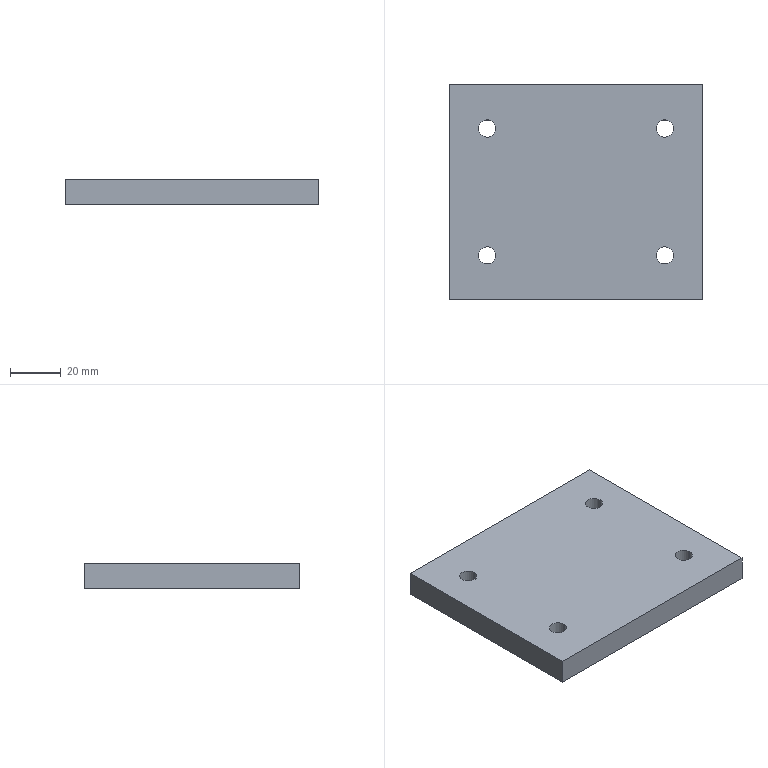Part | SolidWorks | features Extrusion 1, HoleWzd 1 | 1 solid | 14 faces | box 100 x 85 x 10 mm | volume 83547 mm3 | cylinder 8 | plane 6 | commonest cylinder face diameters 6.8 x8
STEP:
#1=CARTESIAN_POINT('',(-31.6,25.,0.));
#2=VERTEX_POINT('',#1);
#3=CARTESIAN_POINT('',(-38.4,25.,0.));
#4=VERTEX_POINT('',#3);
#5=CARTESIAN_POINT('',(-35.,25.,0.));
#6=DIRECTION('',(0.,0.,-1.));
#7=DIRECTION('',(-1.,0.,0.));
#8=AXIS2_PLACEMENT_3D('',#5,#6,#7);
#9=CIRCLE('',#8,3.4);
#10=EDGE_CURVE('',#2,#4,#9,.T.);
#11=ORIENTED_EDGE('',*,*,#10,.T.);
#12=CARTESIAN_POINT('',(-38.4,25.,10.));
#13=VERTEX_POINT('',#12);
#14=CARTESIAN_POINT('',(-38.4,25.,10.));
#15=DIRECTION('',(0.,0.,1.));
#16=VECTOR('',#15,1000.);
#17=LINE('',#14,#16);
#18=EDGE_CURVE('',#4,#13,#17,.T.);
#19=ORIENTED_EDGE('',*,*,#18,.T.);
#20=CARTESIAN_POINT('',(-31.6,25.,10.));
#21=VERTEX_POINT('',#20);
#22=CARTESIAN_POINT('',(-35.,25.,10.));
#23=DIRECTION('',(0.,0.,1.));
#24=DIRECTION('',(1.,0.,0.));
#25=AXIS2_PLACEMENT_3D('',#22,#23,#24);
#26=CIRCLE('',#25,3.4);
#27=EDGE_CURVE('',#13,#21,#26,.T.);
#28=ORIENTED_EDGE('',*,*,#27,.T.);
#29=CARTESIAN_POINT('',(-31.6,25.,10.));
#30=DIRECTION('',(0.,0.,1.));
#31=VECTOR('',#30,1000.);
#32=LINE('',#29,#31);
#33=EDGE_CURVE('',#2,#21,#32,.T.);
#34=ORIENTED_EDGE('',*,*,#33,.F.);
#35=EDGE_LOOP('',(#11,#19,#28,#34));
#36=FACE_OUTER_BOUND('',#35,.T.);
#37=CARTESIAN_POINT('',(-35.,25.,10.));
#38=DIRECTION('',(0.,0.,1.));
#39=DIRECTION('',(1.,0.,0.));
#40=AXIS2_PLACEMENT_3D('',#37,#38,#39);
#41=CYLINDRICAL_SURFACE('',#40,3.4);
#42=ADVANCED_FACE('',(#36),#41,.F.);
#43=CARTESIAN_POINT('',(38.4,25.,0.));
#44=VERTEX_POINT('',#43);
#45=CARTESIAN_POINT('',(31.6,25.,0.));
#46=VERTEX_POINT('',#45);
#47=CARTESIAN_POINT('',(35.,25.,0.));
#48=DIRECTION('',(0.,0.,-1.));
#49=DIRECTION('',(-1.,0.,0.));
#50=AXIS2_PLACEMENT_3D('',#47,#48,#49);
#51=CIRCLE('',#50,3.4);
#52=EDGE_CURVE('',#44,#46,#51,.T.);
#53=ORIENTED_EDGE('',*,*,#52,.T.);
#54=CARTESIAN_POINT('',(31.6,25.,10.));
#55=VERTEX_POINT('',#54);
#56=CARTESIAN_POINT('',(31.6,25.,10.));
#57=DIRECTION('',(0.,0.,1.));
#58=VECTOR('',#57,1000.);
#59=LINE('',#56,#58);
#60=EDGE_CURVE('',#46,#55,#59,.T.);
#61=ORIENTED_EDGE('',*,*,#60,.T.);
#62=CARTESIAN_POINT('',(38.4,25.,10.));
#63=VERTEX_POINT('',#62);
#64=CARTESIAN_POINT('',(35.,25.,10.));
#65=DIRECTION('',(0.,0.,1.));
#66=DIRECTION('',(1.,0.,0.));
#67=AXIS2_PLACEMENT_3D('',#64,#65,#66);
#68=CIRCLE('',#67,3.4);
#69=EDGE_CURVE('',#55,#63,#68,.T.);
#70=ORIENTED_EDGE('',*,*,#69,.T.);
#71=CARTESIAN_POINT('',(38.4,25.,10.));
#72=DIRECTION('',(0.,0.,1.));
#73=VECTOR('',#72,1000.);
#74=LINE('',#71,#73);
#75=EDGE_CURVE('',#44,#63,#74,.T.);
#76=ORIENTED_EDGE('',*,*,#75,.F.);
#77=EDGE_LOOP('',(#53,#61,#70,#76));
#78=FACE_OUTER_BOUND('',#77,.T.);
#79=CARTESIAN_POINT('',(35.,25.,10.));
#80=DIRECTION('',(0.,0.,1.));
#81=DIRECTION('',(1.,0.,0.));
#82=AXIS2_PLACEMENT_3D('',#79,#80,#81);
#83=CYLINDRICAL_SURFACE('',#82,3.4);
#84=ADVANCED_FACE('',(#78),#83,.F.);
#85=CARTESIAN_POINT('',(38.4,-25.,0.));
#86=VERTEX_POINT('',#85);
#87=CARTESIAN_POINT('',(31.6,-25.,0.));
#88=VERTEX_POINT('',#87);
#89=CARTESIAN_POINT('',(35.,-25.,0.));
#90=DIRECTION('',(0.,0.,-1.));
#91=DIRECTION('',(-1.,0.,0.));
#92=AXIS2_PLACEMENT_3D('',#89,#90,#91);
#93=CIRCLE('',#92,3.4);
#94=EDGE_CURVE('',#86,#88,#93,.T.);
#95=ORIENTED_EDGE('',*,*,#94,.T.);
#96=CARTESIAN_POINT('',(31.6,-25.,10.));
#97=VERTEX_POINT('',#96);
#98=CARTESIAN_POINT('',(31.6,-25.,10.));
#99=DIRECTION('',(0.,0.,1.));
#100=VECTOR('',#99,1000.);
#101=LINE('',#98,#100);
#102=EDGE_CURVE('',#88,#97,#101,.T.);
#103=ORIENTED_EDGE('',*,*,#102,.T.);
#104=CARTESIAN_POINT('',(38.4,-25.,10.));
#105=VERTEX_POINT('',#104);
#106=CARTESIAN_POINT('',(35.,-25.,10.));
#107=DIRECTION('',(0.,0.,1.));
#108=DIRECTION('',(1.,0.,0.));
#109=AXIS2_PLACEMENT_3D('',#106,#107,#108);
#110=CIRCLE('',#109,3.4);
#111=EDGE_CURVE('',#97,#105,#110,.T.);
#112=ORIENTED_EDGE('',*,*,#111,.T.);
#113=CARTESIAN_POINT('',(38.4,-25.,10.));
#114=DIRECTION('',(0.,0.,1.));
#115=VECTOR('',#114,1000.);
#116=LINE('',#113,#115);
#117=EDGE_CURVE('',#86,#105,#116,.T.);
#118=ORIENTED_EDGE('',*,*,#117,.F.);
#119=EDGE_LOOP('',(#95,#103,#112,#118));
#120=FACE_OUTER_BOUND('',#119,.T.);
#121=CARTESIAN_POINT('',(35.,-25.,10.));
#122=DIRECTION('',(0.,0.,1.));
#123=DIRECTION('',(1.,0.,0.));
#124=AXIS2_PLACEMENT_3D('',#121,#122,#123);
#125=CYLINDRICAL_SURFACE('',#124,3.4);
#126=ADVANCED_FACE('',(#120),#125,.F.);
#127=CARTESIAN_POINT('',(-31.6,-25.,0.));
#128=VERTEX_POINT('',#127);
#129=CARTESIAN_POINT('',(-38.4,-25.,0.));
#130=VERTEX_POINT('',#129);
#131=CARTESIAN_POINT('',(-35.,-25.,0.));
#132=DIRECTION('',(0.,0.,-1.));
#133=DIRECTION('',(-1.,0.,0.));
#134=AXIS2_PLACEMENT_3D('',#131,#132,#133);
#135=CIRCLE('',#134,3.4);
#136=EDGE_CURVE('',#128,#130,#135,.T.);
#137=ORIENTED_EDGE('',*,*,#136,.T.);
#138=CARTESIAN_POINT('',(-38.4,-25.,10.));
#139=VERTEX_POINT('',#138);
#140=CARTESIAN_POINT('',(-38.4,-25.,10.));
#141=DIRECTION('',(0.,0.,1.));
#142=VECTOR('',#141,1000.);
#143=LINE('',#140,#142);
#144=EDGE_CURVE('',#130,#139,#143,.T.);
#145=ORIENTED_EDGE('',*,*,#144,.T.);
#146=CARTESIAN_POINT('',(-31.6,-25.,10.));
#147=VERTEX_POINT('',#146);
#148=CARTESIAN_POINT('',(-35.,-25.,10.));
#149=DIRECTION('',(0.,0.,1.));
#150=DIRECTION('',(1.,0.,0.));
#151=AXIS2_PLACEMENT_3D('',#148,#149,#150);
#152=CIRCLE('',#151,3.4);
#153=EDGE_CURVE('',#139,#147,#152,.T.);
#154=ORIENTED_EDGE('',*,*,#153,.T.);
#155=CARTESIAN_POINT('',(-31.6,-25.,10.));
#156=DIRECTION('',(0.,0.,1.));
#157=VECTOR('',#156,1000.);
#158=LINE('',#155,#157);
#159=EDGE_CURVE('',#128,#147,#158,.T.);
#160=ORIENTED_EDGE('',*,*,#159,.F.);
#161=EDGE_LOOP('',(#137,#145,#154,#160));
#162=FACE_OUTER_BOUND('',#161,.T.);
#163=CARTESIAN_POINT('',(-35.,-25.,10.));
#164=DIRECTION('',(0.,0.,1.));
#165=DIRECTION('',(1.,0.,0.));
#166=AXIS2_PLACEMENT_3D('',#163,#164,#165);
#167=CYLINDRICAL_SURFACE('',#166,3.4);
#168=ADVANCED_FACE('',(#162),#167,.F.);
#169=CARTESIAN_POINT('',(-50.,42.5,0.));
#170=VERTEX_POINT('',#169);
#171=CARTESIAN_POINT('',(-50.,-42.5,0.));
#172=VERTEX_POINT('',#171);
#173=CARTESIAN_POINT('',(-50.,42.5,0.));
#174=DIRECTION('',(0.,-1.,0.));
#175=VECTOR('',#174,1000.);
#176=LINE('',#173,#175);
#177=EDGE_CURVE('',#170,#172,#176,.T.);
#178=ORIENTED_EDGE('',*,*,#177,.T.);
#179=CARTESIAN_POINT('',(-50.,-42.5,10.));
#180=VERTEX_POINT('',#179);
#181=CARTESIAN_POINT('',(-50.,-42.5,10.));
#182=DIRECTION('',(0.,0.,-1.));
#183=VECTOR('',#182,1000.);
#184=LINE('',#181,#183);
#185=EDGE_CURVE('',#180,#172,#184,.T.);
#186=ORIENTED_EDGE('',*,*,#185,.F.);
#187=CARTESIAN_POINT('',(-50.,42.5,10.));
#188=VERTEX_POINT('',#187);
#189=CARTESIAN_POINT('',(-50.,42.5,10.));
#190=DIRECTION('',(0.,-1.,0.));
#191=VECTOR('',#190,1000.);
#192=LINE('',#189,#191);
#193=EDGE_CURVE('',#188,#180,#192,.T.);
#194=ORIENTED_EDGE('',*,*,#193,.F.);
#195=CARTESIAN_POINT('',(-50.,42.5,10.));
#196=DIRECTION('',(0.,0.,-1.));
#197=VECTOR('',#196,1000.);
#198=LINE('',#195,#197);
#199=EDGE_CURVE('',#188,#170,#198,.T.);
#200=ORIENTED_EDGE('',*,*,#199,.T.);
#201=EDGE_LOOP('',(#178,#186,#194,#200));
#202=FACE_OUTER_BOUND('',#201,.T.);
#203=CARTESIAN_POINT('',(-50.,42.5,10.));
#204=DIRECTION('',(1.,0.,0.));
#205=DIRECTION('',(0.,1.,0.));
#206=AXIS2_PLACEMENT_3D('',#203,#204,#205);
#207=PLANE('',#206);
#208=ADVANCED_FACE('',(#202),#207,.F.);
#209=CARTESIAN_POINT('',(50.,-42.5,0.));
#210=VERTEX_POINT('',#209);
#211=CARTESIAN_POINT('',(50.,-42.5,0.));
#212=DIRECTION('',(1.,0.,0.));
#213=VECTOR('',#212,1000.);
#214=LINE('',#211,#213);
#215=EDGE_CURVE('',#172,#210,#214,.T.);
#216=ORIENTED_EDGE('',*,*,#215,.T.);
#217=CARTESIAN_POINT('',(50.,-42.5,10.));
#218=VERTEX_POINT('',#217);
#219=CARTESIAN_POINT('',(50.,-42.5,10.));
#220=DIRECTION('',(0.,0.,-1.));
#221=VECTOR('',#220,1000.);
#222=LINE('',#219,#221);
#223=EDGE_CURVE('',#218,#210,#222,.T.);
#224=ORIENTED_EDGE('',*,*,#223,.F.);
#225=CARTESIAN_POINT('',(50.,-42.5,10.));
#226=DIRECTION('',(1.,0.,0.));
#227=VECTOR('',#226,1000.);
#228=LINE('',#225,#227);
#229=EDGE_CURVE('',#180,#218,#228,.T.);
#230=ORIENTED_EDGE('',*,*,#229,.F.);
#231=ORIENTED_EDGE('',*,*,#185,.T.);
#232=EDGE_LOOP('',(#216,#224,#230,#231));
#233=FACE_OUTER_BOUND('',#232,.T.);
#234=CARTESIAN_POINT('',(50.,-42.5,10.));
#235=DIRECTION('',(0.,1.,0.));
#236=DIRECTION('',(-1.,0.,0.));
#237=AXIS2_PLACEMENT_3D('',#234,#235,#236);
#238=PLANE('',#237);
#239=ADVANCED_FACE('',(#233),#238,.F.);
#240=CARTESIAN_POINT('',(50.,42.5,0.));
#241=VERTEX_POINT('',#240);
#242=CARTESIAN_POINT('',(50.,42.5,0.));
#243=DIRECTION('',(0.,1.,0.));
#244=VECTOR('',#243,1000.);
#245=LINE('',#242,#244);
#246=EDGE_CURVE('',#210,#241,#245,.T.);
#247=ORIENTED_EDGE('',*,*,#246,.T.);
#248=CARTESIAN_POINT('',(50.,42.5,10.));
#249=VERTEX_POINT('',#248);
#250=CARTESIAN_POINT('',(50.,42.5,10.));
#251=DIRECTION('',(0.,0.,-1.));
#252=VECTOR('',#251,1000.);
#253=LINE('',#250,#252);
#254=EDGE_CURVE('',#249,#241,#253,.T.);
#255=ORIENTED_EDGE('',*,*,#254,.F.);
#256=CARTESIAN_POINT('',(50.,42.5,10.));
#257=DIRECTION('',(0.,1.,0.));
#258=VECTOR('',#257,1000.);
#259=LINE('',#256,#258);
#260=EDGE_CURVE('',#218,#249,#259,.T.);
#261=ORIENTED_EDGE('',*,*,#260,.F.);
#262=ORIENTED_EDGE('',*,*,#223,.T.);
#263=EDGE_LOOP('',(#247,#255,#261,#262));
#264=FACE_OUTER_BOUND('',#263,.T.);
#265=CARTESIAN_POINT('',(50.,42.5,10.));
#266=DIRECTION('',(-1.,0.,0.));
#267=DIRECTION('',(0.,-1.,0.));
#268=AXIS2_PLACEMENT_3D('',#265,#266,#267);
#269=PLANE('',#268);
#270=ADVANCED_FACE('',(#264),#269,.F.);
#271=CARTESIAN_POINT('',(50.,42.5,0.));
#272=DIRECTION('',(-1.,0.,0.));
#273=VECTOR('',#272,1000.);
#274=LINE('',#271,#273);
#275=EDGE_CURVE('',#241,#170,#274,.T.);
#276=ORIENTED_EDGE('',*,*,#275,.T.);
#277=ORIENTED_EDGE('',*,*,#199,.F.);
#278=CARTESIAN_POINT('',(50.,42.5,10.));
#279=DIRECTION('',(-1.,0.,0.));
#280=VECTOR('',#279,1000.);
#281=LINE('',#278,#280);
#282=EDGE_CURVE('',#249,#188,#281,.T.);
#283=ORIENTED_EDGE('',*,*,#282,.F.);
#284=ORIENTED_EDGE('',*,*,#254,.T.);
#285=EDGE_LOOP('',(#276,#277,#283,#284));
#286=FACE_OUTER_BOUND('',#285,.T.);
#287=CARTESIAN_POINT('',(50.,42.5,10.));
#288=DIRECTION('',(0.,-1.,0.));
#289=DIRECTION('',(1.,0.,0.));
#290=AXIS2_PLACEMENT_3D('',#287,#288,#289);
#291=PLANE('',#290);
#292=ADVANCED_FACE('',(#286),#291,.F.);
#293=CARTESIAN_POINT('',(-35.,25.,10.));
#294=DIRECTION('',(0.,0.,1.));
#295=DIRECTION('',(1.,0.,0.));
#296=AXIS2_PLACEMENT_3D('',#293,#294,#295);
#297=CIRCLE('',#296,3.4);
#298=EDGE_CURVE('',#21,#13,#297,.T.);
#299=ORIENTED_EDGE('',*,*,#298,.F.);
#300=ORIENTED_EDGE('',*,*,#27,.F.);
#301=EDGE_LOOP('',(#299,#300));
#302=FACE_BOUND('',#301,.T.);
#303=CARTESIAN_POINT('',(35.,25.,10.));
#304=DIRECTION('',(0.,0.,1.));
#305=DIRECTION('',(1.,0.,0.));
#306=AXIS2_PLACEMENT_3D('',#303,#304,#305);
#307=CIRCLE('',#306,3.4);
#308=EDGE_CURVE('',#63,#55,#307,.T.);
#309=ORIENTED_EDGE('',*,*,#308,.F.);
#310=ORIENTED_EDGE('',*,*,#69,.F.);
#311=EDGE_LOOP('',(#309,#310));
#312=FACE_BOUND('',#311,.T.);
#313=CARTESIAN_POINT('',(35.,-25.,10.));
#314=DIRECTION('',(0.,0.,1.));
#315=DIRECTION('',(1.,0.,0.));
#316=AXIS2_PLACEMENT_3D('',#313,#314,#315);
#317=CIRCLE('',#316,3.4);
#318=EDGE_CURVE('',#105,#97,#317,.T.);
#319=ORIENTED_EDGE('',*,*,#318,.F.);
#320=ORIENTED_EDGE('',*,*,#111,.F.);
#321=EDGE_LOOP('',(#319,#320));
#322=FACE_BOUND('',#321,.T.);
#323=CARTESIAN_POINT('',(-35.,-25.,10.));
#324=DIRECTION('',(0.,0.,1.));
#325=DIRECTION('',(1.,0.,0.));
#326=AXIS2_PLACEMENT_3D('',#323,#324,#325);
#327=CIRCLE('',#326,3.4);
#328=EDGE_CURVE('',#147,#139,#327,.T.);
#329=ORIENTED_EDGE('',*,*,#328,.F.);
#330=ORIENTED_EDGE('',*,*,#153,.F.);
#331=EDGE_LOOP('',(#329,#330));
#332=FACE_BOUND('',#331,.T.);
#333=ORIENTED_EDGE('',*,*,#193,.T.);
#334=ORIENTED_EDGE('',*,*,#229,.T.);
#335=ORIENTED_EDGE('',*,*,#260,.T.);
#336=ORIENTED_EDGE('',*,*,#282,.T.);
#337=EDGE_LOOP('',(#333,#334,#335,#336));
#338=FACE_OUTER_BOUND('',#337,.T.);
#339=CARTESIAN_POINT('',(0.,0.,10.));
#340=DIRECTION('',(0.,0.,-1.));
#341=DIRECTION('',(-1.,0.,0.));
#342=AXIS2_PLACEMENT_3D('',#339,#340,#341);
#343=PLANE('',#342);
#344=ADVANCED_FACE('',(#302,#312,#322,#332,#338),#343,.F.);
#345=ORIENTED_EDGE('',*,*,#10,.F.);
#346=CARTESIAN_POINT('',(-35.,25.,0.));
#347=DIRECTION('',(0.,0.,-1.));
#348=DIRECTION('',(-1.,0.,0.));
#349=AXIS2_PLACEMENT_3D('',#346,#347,#348);
#350=CIRCLE('',#349,3.4);
#351=EDGE_CURVE('',#4,#2,#350,.T.);
#352=ORIENTED_EDGE('',*,*,#351,.F.);
#353=EDGE_LOOP('',(#345,#352));
#354=FACE_BOUND('',#353,.T.);
#355=ORIENTED_EDGE('',*,*,#52,.F.);
#356=CARTESIAN_POINT('',(35.,25.,0.));
#357=DIRECTION('',(0.,0.,-1.));
#358=DIRECTION('',(-1.,0.,0.));
#359=AXIS2_PLACEMENT_3D('',#356,#357,#358);
#360=CIRCLE('',#359,3.4);
#361=EDGE_CURVE('',#46,#44,#360,.T.);
#362=ORIENTED_EDGE('',*,*,#361,.F.);
#363=EDGE_LOOP('',(#355,#362));
#364=FACE_BOUND('',#363,.T.);
#365=ORIENTED_EDGE('',*,*,#94,.F.);
#366=CARTESIAN_POINT('',(35.,-25.,0.));
#367=DIRECTION('',(0.,0.,-1.));
#368=DIRECTION('',(-1.,0.,0.));
#369=AXIS2_PLACEMENT_3D('',#366,#367,#368);
#370=CIRCLE('',#369,3.4);
#371=EDGE_CURVE('',#88,#86,#370,.T.);
#372=ORIENTED_EDGE('',*,*,#371,.F.);
#373=EDGE_LOOP('',(#365,#372));
#374=FACE_BOUND('',#373,.T.);
#375=ORIENTED_EDGE('',*,*,#136,.F.);
#376=CARTESIAN_POINT('',(-35.,-25.,0.));
#377=DIRECTION('',(0.,0.,-1.));
#378=DIRECTION('',(-1.,0.,0.));
#379=AXIS2_PLACEMENT_3D('',#376,#377,#378);
#380=CIRCLE('',#379,3.4);
#381=EDGE_CURVE('',#130,#128,#380,.T.);
#382=ORIENTED_EDGE('',*,*,#381,.F.);
#383=EDGE_LOOP('',(#375,#382));
#384=FACE_BOUND('',#383,.T.);
#385=ORIENTED_EDGE('',*,*,#177,.F.);
#386=ORIENTED_EDGE('',*,*,#275,.F.);
#387=ORIENTED_EDGE('',*,*,#246,.F.);
#388=ORIENTED_EDGE('',*,*,#215,.F.);
#389=EDGE_LOOP('',(#385,#386,#387,#388));
#390=FACE_OUTER_BOUND('',#389,.T.);
#391=CARTESIAN_POINT('',(0.,0.,0.));
#392=DIRECTION('',(0.,0.,-1.));
#393=DIRECTION('',(-1.,0.,0.));
#394=AXIS2_PLACEMENT_3D('',#391,#392,#393);
#395=PLANE('',#394);
#396=ADVANCED_FACE('',(#354,#364,#374,#384,#390),#395,.T.);
#397=ORIENTED_EDGE('',*,*,#144,.F.);
#398=ORIENTED_EDGE('',*,*,#381,.T.);
#399=ORIENTED_EDGE('',*,*,#159,.T.);
#400=ORIENTED_EDGE('',*,*,#328,.T.);
#401=EDGE_LOOP('',(#397,#398,#399,#400));
#402=FACE_OUTER_BOUND('',#401,.T.);
#403=CARTESIAN_POINT('',(-35.,-25.,10.));
#404=DIRECTION('',(0.,0.,1.));
#405=DIRECTION('',(1.,0.,0.));
#406=AXIS2_PLACEMENT_3D('',#403,#404,#405);
#407=CYLINDRICAL_SURFACE('',#406,3.4);
#408=ADVANCED_FACE('',(#402),#407,.F.);
#409=ORIENTED_EDGE('',*,*,#102,.F.);
#410=ORIENTED_EDGE('',*,*,#371,.T.);
#411=ORIENTED_EDGE('',*,*,#117,.T.);
#412=ORIENTED_EDGE('',*,*,#318,.T.);
#413=EDGE_LOOP('',(#409,#410,#411,#412));
#414=FACE_OUTER_BOUND('',#413,.T.);
#415=CARTESIAN_POINT('',(35.,-25.,10.));
#416=DIRECTION('',(0.,0.,1.));
#417=DIRECTION('',(1.,0.,0.));
#418=AXIS2_PLACEMENT_3D('',#415,#416,#417);
#419=CYLINDRICAL_SURFACE('',#418,3.4);
#420=ADVANCED_FACE('',(#414),#419,.F.);
#421=ORIENTED_EDGE('',*,*,#60,.F.);
#422=ORIENTED_EDGE('',*,*,#361,.T.);
#423=ORIENTED_EDGE('',*,*,#75,.T.);
#424=ORIENTED_EDGE('',*,*,#308,.T.);
#425=EDGE_LOOP('',(#421,#422,#423,#424));
#426=FACE_OUTER_BOUND('',#425,.T.);
#427=CARTESIAN_POINT('',(35.,25.,10.));
#428=DIRECTION('',(0.,0.,1.));
#429=DIRECTION('',(1.,0.,0.));
#430=AXIS2_PLACEMENT_3D('',#427,#428,#429);
#431=CYLINDRICAL_SURFACE('',#430,3.4);
#432=ADVANCED_FACE('',(#426),#431,.F.);
#433=ORIENTED_EDGE('',*,*,#18,.F.);
#434=ORIENTED_EDGE('',*,*,#351,.T.);
#435=ORIENTED_EDGE('',*,*,#33,.T.);
#436=ORIENTED_EDGE('',*,*,#298,.T.);
#437=EDGE_LOOP('',(#433,#434,#435,#436));
#438=FACE_OUTER_BOUND('',#437,.T.);
#439=CARTESIAN_POINT('',(-35.,25.,10.));
#440=DIRECTION('',(0.,0.,1.));
#441=DIRECTION('',(1.,0.,0.));
#442=AXIS2_PLACEMENT_3D('',#439,#440,#441);
#443=CYLINDRICAL_SURFACE('',#442,3.4);
#444=ADVANCED_FACE('',(#438),#443,.F.);
#445=CLOSED_SHELL('',(#42,#84,#126,#168,#208,#239,#270,#292,#344,#396,#408,#420,#432,#444));
#446=MANIFOLD_SOLID_BREP('',#445);
#447=CARTESIAN_POINT('',(0.,0.,0.));
#448=DIRECTION('',(0.,0.,1.));
#449=DIRECTION('',(1.,0.,0.));
#450=AXIS2_PLACEMENT_3D('',#447,#448,#449);
#451=(LENGTH_UNIT()NAMED_UNIT(*)SI_UNIT(.MILLI.,.METRE.));
#452=UNCERTAINTY_MEASURE_WITH_UNIT(LENGTH_MEASURE(0.00001),#451,'','');
#453=(NAMED_UNIT(*)PLANE_ANGLE_UNIT()SI_UNIT($,.RADIAN.));
#454=(NAMED_UNIT(*)SI_UNIT($,.STERADIAN.)SOLID_ANGLE_UNIT());
#455=(GEOMETRIC_REPRESENTATION_CONTEXT(3)GLOBAL_UNCERTAINTY_ASSIGNED_CONTEXT((#452))GLOBAL_UNIT_ASSIGNED_CONTEXT((#451,#453,#454))REPRESENTATION_CONTEXT('',''));
#456=ADVANCED_BREP_SHAPE_REPRESENTATION('',(#446,#450),#455);